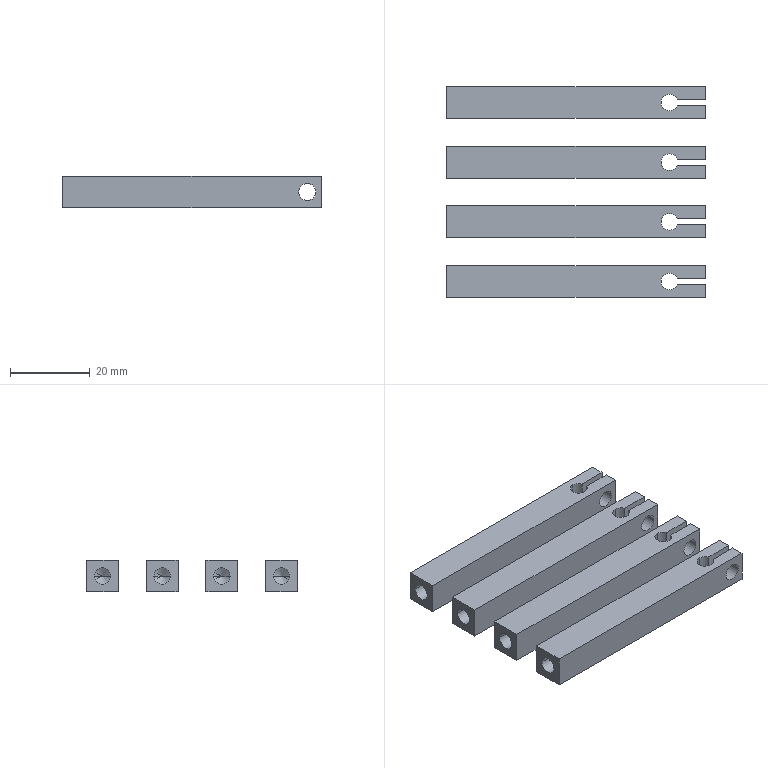NC program | NX | posted with a generic post | part box 65 x 53 x 8 mm
Lines 853 to 3458 of 3458, first 2522 of 2600 lines:
(PLANAR_PROFILE , TOOL : D1.5)
N1692 T13 M6
N1694 G54
N1696 G17 G0 G90 X22.5 Y-34.25 B0. C0. S9500 M3
N1698 G43 Z30. H13
N1700 Z0.9
N1702 G94 G1 Z-0.1 F1000.
N1704 Y-32.5
N1706 Y-25.462
N1708 Y-23.712
N1710 Z0.9
N1712 G0 Z30.
N1714 Z0.8
N1716 G1 Z-0.2
N1718 Y-25.462
N1720 Y-32.5
N1722 Y-34.25
N1724 Z0.8
N1726 G0 Z30.
N1728 Z0.7
N1730 G1 Z-0.3
N1732 Y-32.5
N1734 Y-25.462
N1736 Y-23.712
N1738 Z0.7
N1740 G0 Z30.
N1742 Z0.6
N1744 G1 Z-0.4
N1746 Y-25.462
N1748 Y-32.5
N1750 Y-34.25
N1752 Z0.6
N1754 G0 Z30.
N1756 Z0.5
N1758 G1 Z-0.5
N1760 Y-32.5
N1762 Y-25.462
N1764 Y-23.712
N1766 Z0.5
N1768 G0 Z30.
N1770 Z0.4
N1772 G1 Z-0.6
N1774 Y-25.462
N1776 Y-32.5
N1778 Y-34.25
N1780 Z0.4
N1782 G0 Z30.
N1784 Z0.3
N1786 G1 Z-0.7
N1788 Y-32.5
N1790 Y-25.462
N1792 Y-23.712
N1794 Z0.3
N1796 G0 Z30.
N1798 Z0.2
N1800 G1 Z-0.8
N1802 Y-25.462
N1804 Y-32.5
N1806 Y-34.25
N1808 Z0.2
N1810 G0 Z30.
N1812 Z0.1
N1814 G1 Z-0.9
N1816 Y-32.5
N1818 Y-25.462
N1820 Y-23.712
N1822 Z0.1
N1824 G0 Z30.
N1826 Z0.
N1828 G1 Z-1.
N1830 Y-25.462
N1832 Y-32.5
N1834 Y-34.25
N1836 Z0.
N1838 G0 Z30.
N1840 Z-0.1
N1842 G1 Z-1.1
N1844 Y-32.5
N1846 Y-25.462
N1848 Y-23.712
N1850 Z-0.1
N1852 G0 Z30.
N1854 Z-0.2
N1856 G1 Z-1.2
N1858 Y-25.462
N1860 Y-32.5
N1862 Y-34.25
N1864 Z-0.2
N1866 G0 Z30.
N1868 Z-0.3
N1870 G1 Z-1.3
N1872 Y-32.5
N1874 Y-25.462
N1876 Y-23.712
N1878 Z-0.3
N1880 G0 Z30.
N1882 Z-0.4
N1884 G1 Z-1.4
N1886 Y-25.462
N1888 Y-32.5
N1890 Y-34.25
N1892 Z-0.4
N1894 G0 Z30.
N1896 Z-0.5
N1898 G1 Z-1.5
N1900 Y-32.5
N1902 Y-25.462
N1904 Y-23.712
N1906 Z-0.5
N1908 G0 Z30.
N1910 Z-0.6
N1912 G1 Z-1.6
N1914 Y-25.462
N1916 Y-32.5
N1918 Y-34.25
N1920 Z-0.6
N1922 G0 Z30.
N1924 Z-0.7
N1926 G1 Z-1.7
N1928 Y-32.5
N1930 Y-25.462
N1932 Y-23.712
N1934 Z-0.7
N1936 G0 Z30.
N1938 Z-0.8
N1940 G1 Z-1.8
N1942 Y-25.462
N1944 Y-32.5
N1946 Y-34.25
N1948 Z-0.8
N1950 G0 Z30.
N1952 Z-0.9
N1954 G1 Z-1.9
N1956 Y-32.5
N1958 Y-25.462
N1960 Y-23.712
N1962 Z-0.9
N1964 G0 Z30.
N1966 Z-1.
N1968 G1 Z-2.
N1970 Y-25.462
N1972 Y-32.5
N1974 Y-34.25
N1976 Z-1.
N1978 G0 Z30.
N1980 Z-1.1
N1982 G1 Z-2.1
N1984 Y-32.5
N1986 Y-25.462
N1988 Y-23.712
N1990 Z-1.1
N1992 G0 Z30.
N1994 Z-1.2
N1996 G1 Z-2.2
N1998 Y-25.462
N2000 Y-32.5
N2002 Y-34.25
N2004 Z-1.2
N2006 G0 Z30.
N2008 Z-1.3
N2010 G1 Z-2.3
N2012 Y-32.5
N2014 Y-25.462
N2016 Y-23.712
N2018 Z-1.3
N2020 G0 Z30.
N2022 Z-1.4
N2024 G1 Z-2.4
N2026 Y-25.462
N2028 Y-32.5
N2030 Y-34.25
N2032 Z-1.4
N2034 G0 Z30.
N2036 Z-1.5
N2038 G1 Z-2.5
N2040 Y-32.5
N2042 Y-25.462
N2044 Y-23.712
N2046 Z-1.5
N2048 G0 Z30.
N2050 Z-1.6
N2052 G1 Z-2.6
N2054 Y-25.462
N2056 Y-32.5
N2058 Y-34.25
N2060 Z-1.6
N2062 G0 Z30.
N2064 Z-1.7
N2066 G1 Z-2.7
N2068 Y-32.5
N2070 Y-25.462
N2072 Y-23.712
N2074 Z-1.7
N2076 G0 Z30.
N2078 Z-1.8
N2080 G1 Z-2.8
N2082 Y-25.462
N2084 Y-32.5
N2086 Y-34.25
N2088 Z-1.8
N2090 G0 Z30.
N2092 Z-1.9
N2094 G1 Z-2.9
N2096 Y-32.5
N2098 Y-25.462
N2100 Y-23.712
N2102 Z-1.9
N2104 G0 Z30.
N2106 Z-2.
N2108 G1 Z-3.
N2110 Y-25.462
N2112 Y-32.5
N2114 Y-34.25
N2116 Z-2.
N2118 G0 Z30.
N2120 Z-2.1
N2122 G1 Z-3.1
N2124 Y-32.5
N2126 Y-25.462
N2128 Y-23.712
N2130 Z-2.1
N2132 G0 Z30.
N2134 Z-2.2
N2136 G1 Z-3.2
N2138 Y-25.462
N2140 Y-32.5
N2142 Y-34.25
N2144 Z-2.2
N2146 G0 Z30.
N2148 Z-2.3
N2150 G1 Z-3.3
N2152 Y-32.5
N2154 Y-25.462
N2156 Y-23.712
N2158 Z-2.3
N2160 G0 Z30.
N2162 Z-2.4
N2164 G1 Z-3.4
N2166 Y-25.462
N2168 Y-32.5
N2170 Y-34.25
N2172 Z-2.4
N2174 G0 Z30.
N2176 Z-2.5
N2178 G1 Z-3.5
N2180 Y-32.5
N2182 Y-25.462
N2184 Y-23.712
N2186 Z-2.5
N2188 G0 Z30.
N2190 Z-2.6
N2192 G1 Z-3.6
N2194 Y-25.462
N2196 Y-32.5
N2198 Y-34.25
N2200 Z-2.6
N2202 G0 Z30.
N2204 Z-2.7
N2206 G1 Z-3.7
N2208 Y-32.5
N2210 Y-25.462
N2212 Y-23.712
N2214 Z-2.7
N2216 G0 Z30.
N2218 Z-2.8
N2220 G1 Z-3.8
N2222 Y-25.462
N2224 Y-32.5
N2226 Y-34.25
N2228 Z-2.8
N2230 G0 Z30.
N2232 Z-2.9
N2234 G1 Z-3.9
N2236 Y-32.5
N2238 Y-25.462
N2240 Y-23.712
N2242 Z-2.9
N2244 G0 Z30.
N2246 Z-3.
N2248 G1 Z-4.
N2250 Y-25.462
N2252 Y-32.5
N2254 Y-34.25
N2256 Z-3.
N2258 G0 Z30.
N2260 Z-3.1
N2262 G1 Z-4.1
N2264 Y-32.5
N2266 Y-25.462
N2268 Y-23.712
N2270 Z-3.1
N2272 G0 Z30.
N2274 Z-3.2
N2276 G1 Z-4.2
N2278 Y-25.462
N2280 Y-32.5
N2282 Y-34.25
N2284 Z-3.2
N2286 G0 Z30.
N2288 Z-3.3
N2290 G1 Z-4.3
N2292 Y-32.5
N2294 Y-25.462
N2296 Y-23.712
N2298 Z-3.3
N2300 G0 Z30.
N2302 Z-3.4
N2304 G1 Z-4.4
N2306 Y-25.462
N2308 Y-32.5
N2310 Y-34.25
N2312 Z-3.4
N2314 G0 Z30.
N2316 Z-3.5
N2318 G1 Z-4.5
N2320 Y-32.5
N2322 Y-25.462
N2324 Y-23.712
N2326 Z-3.5
N2328 G0 Z30.
N2330 Z-3.6
N2332 G1 Z-4.6
N2334 Y-25.462
N2336 Y-32.5
N2338 Y-34.25
N2340 Z-3.6
N2342 G0 Z30.
N2344 Z-3.7
N2346 G1 Z-4.7
N2348 Y-32.5
N2350 Y-25.462
N2352 Y-23.712
N2354 Z-3.7
N2356 G0 Z30.
N2358 Z-3.8
N2360 G1 Z-4.8
N2362 Y-25.462
N2364 Y-32.5
N2366 Y-34.25
N2368 Z-3.8
N2370 G0 Z30.
N2372 Z-3.9
N2374 G1 Z-4.9
N2376 Y-32.5
N2378 Y-25.462
N2380 Y-23.712
N2382 Z-3.9
N2384 G0 Z30.
N2386 Z-4.
N2388 G1 Z-5.
N2390 Y-25.462
N2392 Y-32.5
N2394 Y-34.25
N2396 Z-4.
N2398 G0 Z30.
N2400 Z-4.1
N2402 G1 Z-5.1
N2404 Y-32.5
N2406 Y-25.462
N2408 Y-23.712
N2410 Z-4.1
N2412 G0 Z30.
N2414 Z-4.2
N2416 G1 Z-5.2
N2418 Y-25.462
N2420 Y-32.5
N2422 Y-34.25
N2424 Z-4.2
N2426 G0 Z30.
N2428 Z-4.3
N2430 G1 Z-5.3
N2432 Y-32.5
N2434 Y-25.462
N2436 Y-23.712
N2438 Z-4.3
N2440 G0 Z30.
N2442 Z-4.4
N2444 G1 Z-5.4
N2446 Y-25.462
N2448 Y-32.5
N2450 Y-34.25
N2452 Z-4.4
N2454 G0 Z30.
N2456 Z-4.5
N2458 G1 Z-5.5
N2460 Y-32.5
N2462 Y-25.462
N2464 Y-23.712
N2466 Z-4.5
N2468 G0 Z30.
N2470 Z-4.6
N2472 G1 Z-5.6
N2474 Y-25.462
N2476 Y-32.5
N2478 Y-34.25
N2480 Z-4.6
N2482 G0 Z30.
N2484 Z-4.7
N2486 G1 Z-5.7
N2488 Y-32.5
N2490 Y-25.462
N2492 Y-23.712
N2494 Z-4.7
N2496 G0 Z30.
N2498 Z-4.8
N2500 G1 Z-5.8
N2502 Y-25.462
N2504 Y-32.5
N2506 Y-34.25
N2508 Z-4.8
N2510 G0 Z30.
N2512 Z-4.9
N2514 G1 Z-5.9
N2516 Y-32.5
N2518 Y-25.462
N2520 Y-23.712
N2522 Z-4.9
N2524 G0 Z30.
N2526 Z-5.
N2528 G1 Z-6.
N2530 Y-25.462
N2532 Y-32.5
N2534 Y-34.25
N2536 Z-5.
N2538 G0 Z30.
N2540 Z-5.1
N2542 G1 Z-6.1
N2544 Y-32.5
N2546 Y-25.462
N2548 Y-23.712
N2550 Z-5.1
N2552 G0 Z30.
N2554 Z-5.2
N2556 G1 Z-6.2
N2558 Y-25.462
N2560 Y-32.5
N2562 Y-34.25
N2564 Z-5.2
N2566 G0 Z30.
N2568 Z-5.3
N2570 G1 Z-6.3
N2572 Y-32.5
N2574 Y-25.462
N2576 Y-23.712
N2578 Z-5.3
N2580 G0 Z30.
N2582 Z-5.4
N2584 G1 Z-6.4
N2586 Y-25.462
N2588 Y-32.5
N2590 Y-34.25
N2592 Z-5.4
N2594 G0 Z30.
N2596 Z-5.5
N2598 G1 Z-6.5
N2600 Y-32.5
N2602 Y-25.462
N2604 Y-23.712
N2606 Z-5.5
N2608 G0 Z30.
N2610 Z-5.6
N2612 G1 Z-6.6
N2614 Y-25.462
N2616 Y-32.5
N2618 Y-34.25
N2620 Z-5.6
N2622 G0 Z30.
N2624 Z-5.7
N2626 G1 Z-6.7
N2628 Y-32.5
N2630 Y-25.462
N2632 Y-23.712
N2634 Z-5.7
N2636 G0 Z30.
N2638 Z-5.8
N2640 G1 Z-6.8
N2642 Y-25.462
N2644 Y-32.5
N2646 Y-34.25
N2648 Z-5.8
N2650 G0 Z30.
N2652 Z-5.9
N2654 G1 Z-6.9
N2656 Y-32.5
N2658 Y-25.462
N2660 Y-23.712
N2662 Z-5.9
N2664 G0 Z30.
N2666 Z-6.
N2668 G1 Z-7.
N2670 Y-25.462
N2672 Y-32.5
N2674 Y-34.25
N2676 Z-6.
N2678 G0 Z30.
N2680 Z-6.1
N2682 G1 Z-7.1
N2684 Y-32.5
N2686 Y-25.462
N2688 Y-23.712
N2690 Z-6.1
N2692 G0 Z30.
N2694 Z-6.2
N2696 G1 Z-7.2
N2698 Y-25.462
N2700 Y-32.5
N2702 Y-34.25
N2704 Z-6.2
N2706 G0 Z30.
N2708 Z-6.3
N2710 G1 Z-7.3
N2712 Y-32.5
N2714 Y-25.462
N2716 Y-23.712
N2718 Z-6.3
N2720 G0 Z30.
N2722 Z-6.4
N2724 G1 Z-7.4
N2726 Y-25.462
N2728 Y-32.5
N2730 Y-34.25
N2732 Z-6.4
N2734 G0 Z30.
N2736 Z-6.5
N2738 G1 Z-7.5
N2740 Y-32.5
N2742 Y-25.462
N2744 Y-23.712
N2746 Z-6.5
N2748 G0 Z30.
N2750 Z-6.6
N2752 G1 Z-7.6
N2754 Y-25.462
N2756 Y-32.5
N2758 Y-34.25
N2760 Z-6.6
N2762 G0 Z30.
N2764 Z-6.7
N2766 G1 Z-7.7
N2768 Y-32.5
N2770 Y-25.462
N2772 Y-23.712
N2774 Z-6.7
N2776 G0 Z30.
N2778 Z-6.8
N2780 G1 Z-7.8
N2782 Y-25.462
N2784 Y-32.5
N2786 Y-34.25
N2788 Z-6.8
N2790 G0 Z30.
N2792 Z-6.9
N2794 G1 Z-7.9
N2796 Y-32.5
N2798 Y-25.462
N2800 Y-23.712
N2802 Z-6.9
N2804 G0 Z30.
N2806 Z-7.
N2808 G1 Z-8.
N2810 Y-25.462
N2812 Y-32.5
N2814 Y-34.25
N2816 Z-7.
N2818 G0 Z30.
N2820 X7.5
N2822 Z0.9
N2824 G1 Z-0.1
N2826 Y-32.5
N2828 Y-25.462
N2830 Y-23.712
N2832 Z0.9
N2834 G0 Z30.
N2836 Z0.8
N2838 G1 Z-0.2
N2840 Y-25.462
N2842 Y-32.5
N2844 Y-34.25
N2846 Z0.8
N2848 G0 Z30.
N2850 Z0.7
N2852 G1 Z-0.3
N2854 Y-32.5
N2856 Y-25.462
N2858 Y-23.712
N2860 Z0.7
N2862 G0 Z30.
N2864 Z0.6
N2866 G1 Z-0.4
N2868 Y-25.462
N2870 Y-32.5
N2872 Y-34.25
N2874 Z0.6
N2876 G0 Z30.
N2878 Z0.5
N2880 G1 Z-0.5
N2882 Y-32.5
N2884 Y-25.462
N2886 Y-23.712
N2888 Z0.5
N2890 G0 Z30.
N2892 Z0.4
N2894 G1 Z-0.6
N2896 Y-25.462
N2898 Y-32.5
N2900 Y-34.25
N2902 Z0.4
N2904 G0 Z30.
N2906 Z0.3
N2908 G1 Z-0.7
N2910 Y-32.5
N2912 Y-25.462
N2914 Y-23.712
N2916 Z0.3
N2918 G0 Z30.
N2920 Z0.2
N2922 G1 Z-0.8
N2924 Y-25.462
N2926 Y-32.5
N2928 Y-34.25
N2930 Z0.2
N2932 G0 Z30.
N2934 Z0.1
N2936 G1 Z-0.9
N2938 Y-32.5
N2940 Y-25.462
N2942 Y-23.712
N2944 Z0.1
N2946 G0 Z30.
N2948 Z0.
N2950 G1 Z-1.
N2952 Y-25.462
N2954 Y-32.5
N2956 Y-34.25
N2958 Z0.
N2960 G0 Z30.
N2962 Z-0.1
N2964 G1 Z-1.1
N2966 Y-32.5
N2968 Y-25.462
N2970 Y-23.712
N2972 Z-0.1
N2974 G0 Z30.
N2976 Z-0.2
N2978 G1 Z-1.2
N2980 Y-25.462
N2982 Y-32.5
N2984 Y-34.25
N2986 Z-0.2
N2988 G0 Z30.
N2990 Z-0.3
N2992 G1 Z-1.3
N2994 Y-32.5
N2996 Y-25.462
N2998 Y-23.712
N3000 Z-0.3
N3002 G0 Z30.
N3004 Z-0.4
N3006 G1 Z-1.4
N3008 Y-25.462
N3010 Y-32.5
N3012 Y-34.25
N3014 Z-0.4
N3016 G0 Z30.
N3018 Z-0.5
N3020 G1 Z-1.5
N3022 Y-32.5
N3024 Y-25.462
N3026 Y-23.712
N3028 Z-0.5
N3030 G0 Z30.
N3032 Z-0.6
N3034 G1 Z-1.6
N3036 Y-25.462
N3038 Y-32.5
N3040 Y-34.25
N3042 Z-0.6
N3044 G0 Z30.
N3046 Z-0.7
N3048 G1 Z-1.7
N3050 Y-32.5
N3052 Y-25.462
N3054 Y-23.712
N3056 Z-0.7
N3058 G0 Z30.
N3060 Z-0.8
N3062 G1 Z-1.8
N3064 Y-25.462
N3066 Y-32.5
N3068 Y-34.25
N3070 Z-0.8
N3072 G0 Z30.
N3074 Z-0.9
N3076 G1 Z-1.9
N3078 Y-32.5
N3080 Y-25.462
N3082 Y-23.712
N3084 Z-0.9
N3086 G0 Z30.
N3088 Z-1.
N3090 G1 Z-2.
N3092 Y-25.462
N3094 Y-32.5
N3096 Y-34.25
N3098 Z-1.
N3100 G0 Z30.
N3102 Z-1.1
N3104 G1 Z-2.1
N3106 Y-32.5
N3108 Y-25.462
N3110 Y-23.712
N3112 Z-1.1
N3114 G0 Z30.
N3116 Z-1.2
N3118 G1 Z-2.2
N3120 Y-25.462
N3122 Y-32.5
N3124 Y-34.25
N3126 Z-1.2
N3128 G0 Z30.
N3130 Z-1.3
N3132 G1 Z-2.3
N3134 Y-32.5
N3136 Y-25.462
N3138 Y-23.712
N3140 Z-1.3
N3142 G0 Z30.
N3144 Z-1.4
N3146 G1 Z-2.4
N3148 Y-25.462
N3150 Y-32.5
N3152 Y-34.25
N3154 Z-1.4
N3156 G0 Z30.
N3158 Z-1.5
N3160 G1 Z-2.5
N3162 Y-32.5
N3164 Y-25.462
N3166 Y-23.712
N3168 Z-1.5
N3170 G0 Z30.
N3172 Z-1.6
N3174 G1 Z-2.6
N3176 Y-25.462
N3178 Y-32.5
N3180 Y-34.25
N3182 Z-1.6
N3184 G0 Z30.
N3186 Z-1.7
N3188 G1 Z-2.7
N3190 Y-32.5
N3192 Y-25.462
N3194 Y-23.712
N3196 Z-1.7
N3198 G0 Z30.
N3200 Z-1.8
N3202 G1 Z-2.8
N3204 Y-25.462
N3206 Y-32.5
N3208 Y-34.25
N3210 Z-1.8
N3212 G0 Z30.
N3214 Z-1.9
N3216 G1 Z-2.9
N3218 Y-32.5
N3220 Y-25.462
N3222 Y-23.712
N3224 Z-1.9
N3226 G0 Z30.
N3228 Z-2.
N3230 G1 Z-3.
N3232 Y-25.462
N3234 Y-32.5
N3236 Y-34.25
N3238 Z-2.
N3240 G0 Z30.
N3242 Z-2.1
N3244 G1 Z-3.1
N3246 Y-32.5
N3248 Y-25.462
N3250 Y-23.712
N3252 Z-2.1
N3254 G0 Z30.
N3256 Z-2.2
N3258 G1 Z-3.2
N3260 Y-25.462
N3262 Y-32.5
N3264 Y-34.25
N3266 Z-2.2
N3268 G0 Z30.
N3270 Z-2.3
N3272 G1 Z-3.3
N3274 Y-32.5
N3276 Y-25.462
N3278 Y-23.712
N3280 Z-2.3
N3282 G0 Z30.
N3284 Z-2.4
N3286 G1 Z-3.4
N3288 Y-25.462
N3290 Y-32.5
N3292 Y-34.25
N3294 Z-2.4
N3296 G0 Z30.
N3298 Z-2.5
N3300 G1 Z-3.5
N3302 Y-32.5
N3304 Y-25.462
N3306 Y-23.712
N3308 Z-2.5
N3310 G0 Z30.
N3312 Z-2.6
N3314 G1 Z-3.6
N3316 Y-25.462
N3318 Y-32.5
N3320 Y-34.25
N3322 Z-2.6
N3324 G0 Z30.
N3326 Z-2.7
N3328 G1 Z-3.7
N3330 Y-32.5
N3332 Y-25.462
N3334 Y-23.712
N3336 Z-2.7
N3338 G0 Z30.
N3340 Z-2.8
N3342 G1 Z-3.8
N3344 Y-25.462
N3346 Y-32.5
N3348 Y-34.25
N3350 Z-2.8
N3352 G0 Z30.
N3354 Z-2.9
N3356 G1 Z-3.9
N3358 Y-32.5
N3360 Y-25.462
N3362 Y-23.712
N3364 Z-2.9
N3366 G0 Z30.
N3368 Z-3.
N3370 G1 Z-4.
N3372 Y-25.462
N3374 Y-32.5
N3376 Y-34.25
N3378 Z-3.
N3380 G0 Z30.
N3382 Z-3.1
N3384 G1 Z-4.1
N3386 Y-32.5
N3388 Y-25.462
N3390 Y-23.712
N3392 Z-3.1
N3394 G0 Z30.
N3396 Z-3.2
N3398 G1 Z-4.2
N3400 Y-25.462
N3402 Y-32.5
N3404 Y-34.25
N3406 Z-3.2
N3408 G0 Z30.
N3410 Z-3.3
N3412 G1 Z-4.3
N3414 Y-32.5
N3416 Y-25.462
N3418 Y-23.712
N3420 Z-3.3
N3422 G0 Z30.
N3424 Z-3.4
N3426 G1 Z-4.4
N3428 Y-25.462
N3430 Y-32.5
N3432 Y-34.25
N3434 Z-3.4
N3436 G0 Z30.
N3438 Z-3.5
N3440 G1 Z-4.5
N3442 Y-32.5
N3444 Y-25.462
N3446 Y-23.712
N3448 Z-3.5
N3450 G0 Z30.
N3452 Z-3.6
N3454 G1 Z-4.6
N3456 Y-25.462
N3458 Y-32.5
N3460 Y-34.25
N3462 Z-3.6
N3464 G0 Z30.
N3466 Z-3.7
N3468 G1 Z-4.7
N3470 Y-32.5
N3472 Y-25.462
N3474 Y-23.712
N3476 Z-3.7
N3478 G0 Z30.
N3480 Z-3.8
N3482 G1 Z-4.8
N3484 Y-25.462
N3486 Y-32.5
N3488 Y-34.25
N3490 Z-3.8
N3492 G0 Z30.
N3494 Z-3.9
N3496 G1 Z-4.9
N3498 Y-32.5
N3500 Y-25.462
N3502 Y-23.712
N3504 Z-3.9
N3506 G0 Z30.
N3508 Z-4.
N3510 G1 Z-5.
N3512 Y-25.462
N3514 Y-32.5
N3516 Y-34.25
N3518 Z-4.
N3520 G0 Z30.
N3522 Z-4.1
N3524 G1 Z-5.1
N3526 Y-32.5
N3528 Y-25.462
N3530 Y-23.712
N3532 Z-4.1
N3534 G0 Z30.
N3536 Z-4.2
N3538 G1 Z-5.2
N3540 Y-25.462
N3542 Y-32.5
N3544 Y-34.25
N3546 Z-4.2
N3548 G0 Z30.
N3550 Z-4.3
N3552 G1 Z-5.3
N3554 Y-32.5
N3556 Y-25.462
N3558 Y-23.712
N3560 Z-4.3
N3562 G0 Z30.
N3564 Z-4.4
N3566 G1 Z-5.4
N3568 Y-25.462
N3570 Y-32.5
N3572 Y-34.25
N3574 Z-4.4
N3576 G0 Z30.
N3578 Z-4.5
N3580 G1 Z-5.5
N3582 Y-32.5
N3584 Y-25.462
N3586 Y-23.712
N3588 Z-4.5
N3590 G0 Z30.
N3592 Z-4.6
N3594 G1 Z-5.6
N3596 Y-25.462
N3598 Y-32.5
N3600 Y-34.25
N3602 Z-4.6
N3604 G0 Z30.
N3606 Z-4.7
N3608 G1 Z-5.7
N3610 Y-32.5
N3612 Y-25.462
N3614 Y-23.712
N3616 Z-4.7
N3618 G0 Z30.
N3620 Z-4.8
N3622 G1 Z-5.8
N3624 Y-25.462
N3626 Y-32.5
N3628 Y-34.25
N3630 Z-4.8
N3632 G0 Z30.
N3634 Z-4.9
N3636 G1 Z-5.9
N3638 Y-32.5
N3640 Y-25.462
N3642 Y-23.712
N3644 Z-4.9
N3646 G0 Z30.
N3648 Z-5.
N3650 G1 Z-6.
N3652 Y-25.462
N3654 Y-32.5
N3656 Y-34.25
N3658 Z-5.
N3660 G0 Z30.
N3662 Z-5.1
N3664 G1 Z-6.1
N3666 Y-32.5
N3668 Y-25.462
N3670 Y-23.712
N3672 Z-5.1
N3674 G0 Z30.
N3676 Z-5.2
N3678 G1 Z-6.2
N3680 Y-25.462
N3682 Y-32.5
N3684 Y-34.25
N3686 Z-5.2
N3688 G0 Z30.
N3690 Z-5.3
N3692 G1 Z-6.3
N3694 Y-32.5
N3696 Y-25.462
N3698 Y-23.712
N3700 Z-5.3
N3702 G0 Z30.
N3704 Z-5.4
N3706 G1 Z-6.4
N3708 Y-25.462
N3710 Y-32.5
N3712 Y-34.25
N3714 Z-5.4
N3716 G0 Z30.
N3718 Z-5.5
N3720 G1 Z-6.5
N3722 Y-32.5
N3724 Y-25.462
N3726 Y-23.712
N3728 Z-5.5
N3730 G0 Z30.
N3732 Z-5.6
N3734 G1 Z-6.6
N3736 Y-25.462
N3738 Y-32.5
N3740 Y-34.25
N3742 Z-5.6
N3744 G0 Z30.
N3746 Z-5.7
N3748 G1 Z-6.7
N3750 Y-32.5
N3752 Y-25.462
N3754 Y-23.712
N3756 Z-5.7
N3758 G0 Z30.
N3760 Z-5.8
N3762 G1 Z-6.8
N3764 Y-25.462
N3766 Y-32.5
N3768 Y-34.25
N3770 Z-5.8
N3772 G0 Z30.
N3774 Z-5.9
N3776 G1 Z-6.9
N3778 Y-32.5
N3780 Y-25.462
N3782 Y-23.712
N3784 Z-5.9
N3786 G0 Z30.
N3788 Z-6.
N3790 G1 Z-7.
N3792 Y-25.462
N3794 Y-32.5
N3796 Y-34.25
N3798 Z-6.
N3800 G0 Z30.
N3802 Z-6.1
N3804 G1 Z-7.1
N3806 Y-32.5
N3808 Y-25.462
N3810 Y-23.712
N3812 Z-6.1
N3814 G0 Z30.
N3816 Z-6.2
N3818 G1 Z-7.2
N3820 Y-25.462
N3822 Y-32.5
N3824 Y-34.25
N3826 Z-6.2
N3828 G0 Z30.
N3830 Z-6.3
N3832 G1 Z-7.3
N3834 Y-32.5
N3836 Y-25.462
N3838 Y-23.712
N3840 Z-6.3
N3842 G0 Z30.
N3844 Z-6.4
N3846 G1 Z-7.4
N3848 Y-25.462
N3850 Y-32.5
N3852 Y-34.25
N3854 Z-6.4
N3856 G0 Z30.
N3858 Z-6.5
N3860 G1 Z-7.5
N3862 Y-32.5
N3864 Y-25.462
N3866 Y-23.712
N3868 Z-6.5
N3870 G0 Z30.
N3872 Z-6.6
N3874 G1 Z-7.6
N3876 Y-25.462
N3878 Y-32.5
N3880 Y-34.25
N3882 Z-6.6
N3884 G0 Z30.
N3886 Z-6.7
N3888 G1 Z-7.7
N3890 Y-32.5
N3892 Y-25.462
N3894 Y-23.712
N3896 Z-6.7
N3898 G0 Z30.
N3900 Z-6.8
N3902 G1 Z-7.8
N3904 Y-25.462
N3906 Y-32.5
N3908 Y-34.25
N3910 Z-6.8
N3912 G0 Z30.
N3914 Z-6.9
N3916 G1 Z-7.9
N3918 Y-32.5
N3920 Y-25.462
N3922 Y-23.712
N3924 Z-6.9
N3926 G0 Z30.
N3928 Z-7.
N3930 G1 Z-8.
N3932 Y-25.462
N3934 Y-32.5
N3936 Y-34.25
N3938 Z-7.
N3940 G0 Z30.
N3942 X-7.5
N3944 Z0.9
N3946 G1 Z-0.1
N3948 Y-32.5
N3950 Y-25.462
N3952 Y-23.712
N3954 Z0.9
N3956 G0 Z30.
N3958 Z0.8
N3960 G1 Z-0.2
N3962 Y-25.462
N3964 Y-32.5
N3966 Y-34.25
N3968 Z0.8
N3970 G0 Z30.
N3972 Z0.7
N3974 G1 Z-0.3
N3976 Y-32.5
N3978 Y-25.462
N3980 Y-23.712
N3982 Z0.7
N3984 G0 Z30.
N3986 Z0.6
N3988 G1 Z-0.4
N3990 Y-25.462
N3992 Y-32.5
N3994 Y-34.25
N3996 Z0.6
N3998 G0 Z30.
N4000 Z0.5
N4002 G1 Z-0.5
N4004 Y-32.5
N4006 Y-25.462
N4008 Y-23.712
N4010 Z0.5
N4012 G0 Z30.
N4014 Z0.4
N4016 G1 Z-0.6
N4018 Y-25.462
N4020 Y-32.5
N4022 Y-34.25
N4024 Z0.4
N4026 G0 Z30.
N4028 Z0.3
N4030 G1 Z-0.7
N4032 Y-32.5
N4034 Y-25.462
N4036 Y-23.712
N4038 Z0.3
N4040 G0 Z30.
N4042 Z0.2
N4044 G1 Z-0.8
N4046 Y-25.462
N4048 Y-32.5
N4050 Y-34.25
N4052 Z0.2
N4054 G0 Z30.
N4056 Z0.1
N4058 G1 Z-0.9
N4060 Y-32.5
N4062 Y-25.462
N4064 Y-23.712
N4066 Z0.1
N4068 G0 Z30.
N4070 Z0.
N4072 G1 Z-1.
N4074 Y-25.462
N4076 Y-32.5
N4078 Y-34.25
N4080 Z0.
N4082 G0 Z30.
N4084 Z-0.1
N4086 G1 Z-1.1
N4088 Y-32.5
N4090 Y-25.462
N4092 Y-23.712
N4094 Z-0.1
N4096 G0 Z30.
N4098 Z-0.2
N4100 G1 Z-1.2
N4102 Y-25.462
N4104 Y-32.5
N4106 Y-34.25
N4108 Z-0.2
N4110 G0 Z30.
N4112 Z-0.3
N4114 G1 Z-1.3
N4116 Y-32.5
N4118 Y-25.462
N4120 Y-23.712
N4122 Z-0.3
N4124 G0 Z30.
N4126 Z-0.4
N4128 G1 Z-1.4
N4130 Y-25.462
N4132 Y-32.5
N4134 Y-34.25
N4136 Z-0.4
N4138 G0 Z30.
N4140 Z-0.5
N4142 G1 Z-1.5
N4144 Y-32.5
N4146 Y-25.462
N4148 Y-23.712
N4150 Z-0.5
N4152 G0 Z30.
N4154 Z-0.6
N4156 G1 Z-1.6
N4158 Y-25.462
N4160 Y-32.5
N4162 Y-34.25
N4164 Z-0.6
N4166 G0 Z30.
N4168 Z-0.7
N4170 G1 Z-1.7
N4172 Y-32.5
N4174 Y-25.462
N4176 Y-23.712
N4178 Z-0.7
N4180 G0 Z30.
N4182 Z-0.8
N4184 G1 Z-1.8
N4186 Y-25.462
N4188 Y-32.5
N4190 Y-34.25
N4192 Z-0.8
N4194 G0 Z30.
N4196 Z-0.9
N4198 G1 Z-1.9
N4200 Y-32.5
N4202 Y-25.462
N4204 Y-23.712
N4206 Z-0.9
N4208 G0 Z30.
N4210 Z-1.
N4212 G1 Z-2.
N4214 Y-25.462
N4216 Y-32.5
N4218 Y-34.25
N4220 Z-1.
N4222 G0 Z30.
N4224 Z-1.1
N4226 G1 Z-2.1
N4228 Y-32.5
N4230 Y-25.462
N4232 Y-23.712
N4234 Z-1.1
N4236 G0 Z30.
N4238 Z-1.2
N4240 G1 Z-2.2
N4242 Y-25.462
N4244 Y-32.5
N4246 Y-34.25
N4248 Z-1.2
N4250 G0 Z30.
N4252 Z-1.3
N4254 G1 Z-2.3
N4256 Y-32.5
N4258 Y-25.462
N4260 Y-23.712
N4262 Z-1.3
N4264 G0 Z30.
N4266 Z-1.4
N4268 G1 Z-2.4
N4270 Y-25.462
N4272 Y-32.5
N4274 Y-34.25
N4276 Z-1.4
N4278 G0 Z30.
N4280 Z-1.5
N4282 G1 Z-2.5
N4284 Y-32.5
N4286 Y-25.462
N4288 Y-23.712
N4290 Z-1.5
N4292 G0 Z30.
N4294 Z-1.6
N4296 G1 Z-2.6
N4298 Y-25.462
N4300 Y-32.5
N4302 Y-34.25
N4304 Z-1.6
N4306 G0 Z30.
N4308 Z-1.7
N4310 G1 Z-2.7
N4312 Y-32.5
N4314 Y-25.462
N4316 Y-23.712
N4318 Z-1.7
N4320 G0 Z30.
N4322 Z-1.8
N4324 G1 Z-2.8
N4326 Y-25.462
N4328 Y-32.5
N4330 Y-34.25
N4332 Z-1.8
N4334 G0 Z30.
N4336 Z-1.9
N4338 G1 Z-2.9
N4340 Y-32.5
N4342 Y-25.462
N4344 Y-23.712
N4346 Z-1.9
N4348 G0 Z30.
N4350 Z-2.
N4352 G1 Z-3.
N4354 Y-25.462
N4356 Y-32.5
N4358 Y-34.25
N4360 Z-2.
N4362 G0 Z30.
N4364 Z-2.1
N4366 G1 Z-3.1
N4368 Y-32.5
N4370 Y-25.462
N4372 Y-23.712
N4374 Z-2.1
N4376 G0 Z30.
N4378 Z-2.2
N4380 G1 Z-3.2
N4382 Y-25.462
N4384 Y-32.5
N4386 Y-34.25
N4388 Z-2.2
N4390 G0 Z30.
N4392 Z-2.3
N4394 G1 Z-3.3
N4396 Y-32.5
N4398 Y-25.462
N4400 Y-23.712
N4402 Z-2.3
N4404 G0 Z30.
N4406 Z-2.4
N4408 G1 Z-3.4
N4410 Y-25.462
N4412 Y-32.5
N4414 Y-34.25
N4416 Z-2.4
N4418 G0 Z30.
N4420 Z-2.5
N4422 G1 Z-3.5
N4424 Y-32.5
N4426 Y-25.462
N4428 Y-23.712
N4430 Z-2.5
N4432 G0 Z30.
N4434 Z-2.6
N4436 G1 Z-3.6
N4438 Y-25.462
N4440 Y-32.5
N4442 Y-34.25
N4444 Z-2.6
N4446 G0 Z30.
N4448 Z-2.7
N4450 G1 Z-3.7
N4452 Y-32.5
N4454 Y-25.462
N4456 Y-23.712
N4458 Z-2.7
N4460 G0 Z30.
N4462 Z-2.8
N4464 G1 Z-3.8
N4466 Y-25.462
N4468 Y-32.5
N4470 Y-34.25
N4472 Z-2.8
N4474 G0 Z30.
N4476 Z-2.9
N4478 G1 Z-3.9
N4480 Y-32.5
N4482 Y-25.462
N4484 Y-23.712
N4486 Z-2.9
N4488 G0 Z30.
N4490 Z-3.
N4492 G1 Z-4.
N4494 Y-25.462
N4496 Y-32.5
N4498 Y-34.25
N4500 Z-3.
N4502 G0 Z30.
N4504 Z-3.1
N4506 G1 Z-4.1
N4508 Y-32.5
N4510 Y-25.462
N4512 Y-23.712
N4514 Z-3.1
N4516 G0 Z30.
N4518 Z-3.2
N4520 G1 Z-4.2
N4522 Y-25.462
N4524 Y-32.5
N4526 Y-34.25
N4528 Z-3.2
N4530 G0 Z30.
N4532 Z-3.3
N4534 G1 Z-4.3
N4536 Y-32.5
N4538 Y-25.462
N4540 Y-23.712
N4542 Z-3.3
N4544 G0 Z30.
N4546 Z-3.4
N4548 G1 Z-4.4
N4550 Y-25.462
N4552 Y-32.5
N4554 Y-34.25
N4556 Z-3.4
N4558 G0 Z30.
N4560 Z-3.5
N4562 G1 Z-4.5
N4564 Y-32.5
N4566 Y-25.462
N4568 Y-23.712
N4570 Z-3.5
N4572 G0 Z30.
N4574 Z-3.6
N4576 G1 Z-4.6
N4578 Y-25.462
N4580 Y-32.5
N4582 Y-34.25
N4584 Z-3.6
N4586 G0 Z30.
N4588 Z-3.7
N4590 G1 Z-4.7
N4592 Y-32.5
N4594 Y-25.462
N4596 Y-23.712
N4598 Z-3.7
N4600 G0 Z30.
N4602 Z-3.8
N4604 G1 Z-4.8
N4606 Y-25.462
N4608 Y-32.5
N4610 Y-34.25
N4612 Z-3.8
N4614 G0 Z30.
N4616 Z-3.9
N4618 G1 Z-4.9
N4620 Y-32.5
N4622 Y-25.462
N4624 Y-23.712
N4626 Z-3.9
N4628 G0 Z30.
N4630 Z-4.
N4632 G1 Z-5.
N4634 Y-25.462
N4636 Y-32.5
N4638 Y-34.25
N4640 Z-4.
N4642 G0 Z30.
N4644 Z-4.1
N4646 G1 Z-5.1
N4648 Y-32.5
N4650 Y-25.462
N4652 Y-23.712
N4654 Z-4.1
N4656 G0 Z30.
N4658 Z-4.2
N4660 G1 Z-5.2
N4662 Y-25.462
N4664 Y-32.5
N4666 Y-34.25
N4668 Z-4.2
N4670 G0 Z30.
N4672 Z-4.3
N4674 G1 Z-5.3
N4676 Y-32.5
N4678 Y-25.462
N4680 Y-23.712
N4682 Z-4.3
N4684 G0 Z30.
N4686 Z-4.4
N4688 G1 Z-5.4
N4690 Y-25.462
N4692 Y-32.5
N4694 Y-34.25
N4696 Z-4.4
N4698 G0 Z30.
N4700 Z-4.5
N4702 G1 Z-5.5
N4704 Y-32.5
N4706 Y-25.462
N4708 Y-23.712
N4710 Z-4.5
N4712 G0 Z30.
N4714 Z-4.6
N4716 G1 Z-5.6
N4718 Y-25.462
N4720 Y-32.5
N4722 Y-34.25
N4724 Z-4.6
N4726 G0 Z30.
N4728 Z-4.7
N4730 G1 Z-5.7
N4732 Y-32.5
N4734 Y-25.462
N4736 Y-23.712
N4738 Z-4.7
N4740 G0 Z30.
N4742 Z-4.8
N4744 G1 Z-5.8
N4746 Y-25.462
N4748 Y-32.5
N4750 Y-34.25
N4752 Z-4.8
N4754 G0 Z30.
N4756 Z-4.9
N4758 G1 Z-5.9
N4760 Y-32.5
N4762 Y-25.462
N4764 Y-23.712
N4766 Z-4.9
N4768 G0 Z30.
N4770 Z-5.
N4772 G1 Z-6.
N4774 Y-25.462
N4776 Y-32.5
N4778 Y-34.25
N4780 Z-5.
N4782 G0 Z30.
N4784 Z-5.1
N4786 G1 Z-6.1
N4788 Y-32.5
N4790 Y-25.462
N4792 Y-23.712
N4794 Z-5.1
N4796 G0 Z30.
N4798 Z-5.2
N4800 G1 Z-6.2
N4802 Y-25.462
N4804 Y-32.5
N4806 Y-34.25
N4808 Z-5.2
N4810 G0 Z30.
N4812 Z-5.3
N4814 G1 Z-6.3
N4816 Y-32.5
N4818 Y-25.462
N4820 Y-23.712
N4822 Z-5.3
N4824 G0 Z30.
N4826 Z-5.4
N4828 G1 Z-6.4
N4830 Y-25.462
N4832 Y-32.5
N4834 Y-34.25
N4836 Z-5.4
N4838 G0 Z30.
N4840 Z-5.5
N4842 G1 Z-6.5
N4844 Y-32.5
N4846 Y-25.462
N4848 Y-23.712
N4850 Z-5.5
N4852 G0 Z30.
N4854 Z-5.6
N4856 G1 Z-6.6
N4858 Y-25.462
N4860 Y-32.5
N4862 Y-34.25
N4864 Z-5.6
N4866 G0 Z30.
N4868 Z-5.7
N4870 G1 Z-6.7
N4872 Y-32.5
N4874 Y-25.462
N4876 Y-23.712
N4878 Z-5.7
N4880 G0 Z30.
N4882 Z-5.8
N4884 G1 Z-6.8
N4886 Y-25.462
N4888 Y-32.5
N4890 Y-34.25
N4892 Z-5.8
N4894 G0 Z30.
N4896 Z-5.9
N4898 G1 Z-6.9
N4900 Y-32.5
N4902 Y-25.462
N4904 Y-23.712
N4906 Z-5.9
N4908 G0 Z30.
N4910 Z-6.
N4912 G1 Z-7.
N4914 Y-25.462
N4916 Y-32.5
N4918 Y-34.25
N4920 Z-6.
N4922 G0 Z30.
N4924 Z-6.1
N4926 G1 Z-7.1
N4928 Y-32.5
N4930 Y-25.462
N4932 Y-23.712
N4934 Z-6.1
N4936 G0 Z30.
N4938 Z-6.2
N4940 G1 Z-7.2
N4942 Y-25.462
N4944 Y-32.5
N4946 Y-34.25
N4948 Z-6.2
N4950 G0 Z30.
N4952 Z-6.3
N4954 G1 Z-7.3
N4956 Y-32.5
N4958 Y-25.462
N4960 Y-23.712
N4962 Z-6.3
N4964 G0 Z30.
N4966 Z-6.4
N4968 G1 Z-7.4
N4970 Y-25.462
N4972 Y-32.5
N4974 Y-34.25
N4976 Z-6.4
N4978 G0 Z30.
N4980 Z-6.5
N4982 G1 Z-7.5
N4984 Y-32.5
N4986 Y-25.462
N4988 Y-23.712
N4990 Z-6.5
N4992 G0 Z30.
N4994 Z-6.6
N4996 G1 Z-7.6
N4998 Y-25.462
N5000 Y-32.5
N5002 Y-34.25
N5004 Z-6.6
N5006 G0 Z30.
N5008 Z-6.7
N5010 G1 Z-7.7
N5012 Y-32.5
N5014 Y-25.462
N5016 Y-23.712
N5018 Z-6.7
N5020 G0 Z30.
N5022 Z-6.8
N5024 G1 Z-7.8
N5026 Y-25.462
N5028 Y-32.5
N5030 Y-34.25
N5032 Z-6.8
N5034 G0 Z30.
N5036 Z-6.9
N5038 G1 Z-7.9
N5040 Y-32.5
N5042 Y-25.462
N5044 Y-23.712
N5046 Z-6.9
N5048 G0 Z30.
N5050 Z-7.
N5052 G1 Z-8.
N5054 Y-25.462
N5056 Y-32.5
N5058 Y-34.25
N5060 Z-7.
N5062 G0 Z30.
N5064 X-22.5
N5066 Z0.9
N5068 G1 Z-0.1
N5070 Y-32.5
N5072 Y-25.462
N5074 Y-23.712
N5076 Z0.9
N5078 G0 Z30.
N5080 Z0.8
N5082 G1 Z-0.2
N5084 Y-25.462
N5086 Y-32.5
N5088 Y-34.25
N5090 Z0.8
N5092 G0 Z30.
N5094 Z0.7
N5096 G1 Z-0.3
N5098 Y-32.5
N5100 Y-25.462
N5102 Y-23.712
N5104 Z0.7
N5106 G0 Z30.
N5108 Z0.6
N5110 G1 Z-0.4
N5112 Y-25.462
N5114 Y-32.5
N5116 Y-34.25
N5118 Z0.6
N5120 G0 Z30.
N5122 Z0.5
N5124 G1 Z-0.5
N5126 Y-32.5
N5128 Y-25.462
N5130 Y-23.712
N5132 Z0.5
N5134 G0 Z30.
N5136 Z0.4
N5138 G1 Z-0.6
N5140 Y-25.462
N5142 Y-32.5
N5144 Y-34.25
N5146 Z0.4
N5148 G0 Z30.
N5150 Z0.3
N5152 G1 Z-0.7
N5154 Y-32.5
N5156 Y-25.462
N5158 Y-23.712
N5160 Z0.3
N5162 G0 Z30.
N5164 Z0.2
N5166 G1 Z-0.8
N5168 Y-25.462
N5170 Y-32.5
N5172 Y-34.25
N5174 Z0.2
N5176 G0 Z30.
N5178 Z0.1
N5180 G1 Z-0.9
N5182 Y-32.5
N5184 Y-25.462
N5186 Y-23.712
N5188 Z0.1
N5190 G0 Z30.
N5192 Z0.
N5194 G1 Z-1.
N5196 Y-25.462
N5198 Y-32.5
N5200 Y-34.25
N5202 Z0.
N5204 G0 Z30.
N5206 Z-0.1
N5208 G1 Z-1.1
N5210 Y-32.5
N5212 Y-25.462
N5214 Y-23.712
N5216 Z-0.1
N5218 G0 Z30.
N5220 Z-0.2
N5222 G1 Z-1.2
N5224 Y-25.462
N5226 Y-32.5
N5228 Y-34.25
N5230 Z-0.2
N5232 G0 Z30.
N5234 Z-0.3
N5236 G1 Z-1.3
N5238 Y-32.5
N5240 Y-25.462
N5242 Y-23.712
N5244 Z-0.3
N5246 G0 Z30.
N5248 Z-0.4
N5250 G1 Z-1.4
N5252 Y-25.462
N5254 Y-32.5
N5256 Y-34.25
N5258 Z-0.4
N5260 G0 Z30.
N5262 Z-0.5
N5264 G1 Z-1.5
N5266 Y-32.5
N5268 Y-25.462
N5270 Y-23.712
N5272 Z-0.5
N5274 G0 Z30.
N5276 Z-0.6
N5278 G1 Z-1.6
N5280 Y-25.462
N5282 Y-32.5
N5284 Y-34.25
N5286 Z-0.6
N5288 G0 Z30.
N5290 Z-0.7
N5292 G1 Z-1.7
N5294 Y-32.5
N5296 Y-25.462
N5298 Y-23.712
N5300 Z-0.7
N5302 G0 Z30.
N5304 Z-0.8
N5306 G1 Z-1.8
N5308 Y-25.462
N5310 Y-32.5
N5312 Y-34.25
N5314 Z-0.8
N5316 G0 Z30.
N5318 Z-0.9
N5320 G1 Z-1.9
N5322 Y-32.5
N5324 Y-25.462
N5326 Y-23.712
N5328 Z-0.9
N5330 G0 Z30.
N5332 Z-1.
N5334 G1 Z-2.
N5336 Y-25.462
N5338 Y-32.5
N5340 Y-34.25
N5342 Z-1.
N5344 G0 Z30.
N5346 Z-1.1
N5348 G1 Z-2.1
N5350 Y-32.5
N5352 Y-25.462
N5354 Y-23.712
N5356 Z-1.1
N5358 G0 Z30.
N5360 Z-1.2
N5362 G1 Z-2.2
N5364 Y-25.462
N5366 Y-32.5
N5368 Y-34.25
N5370 Z-1.2
N5372 G0 Z30.
N5374 Z-1.3
N5376 G1 Z-2.3
N5378 Y-32.5
N5380 Y-25.462
N5382 Y-23.712
N5384 Z-1.3
N5386 G0 Z30.
N5388 Z-1.4
N5390 G1 Z-2.4
N5392 Y-25.462
N5394 Y-32.5
N5396 Y-34.25
N5398 Z-1.4
N5400 G0 Z30.
N5402 Z-1.5
N5404 G1 Z-2.5
N5406 Y-32.5
N5408 Y-25.462
N5410 Y-23.712
N5412 Z-1.5
N5414 G0 Z30.
N5416 Z-1.6
N5418 G1 Z-2.6
N5420 Y-25.462
N5422 Y-32.5
N5424 Y-34.25
N5426 Z-1.6
N5428 G0 Z30.
N5430 Z-1.7
N5432 G1 Z-2.7
N5434 Y-32.5
N5436 Y-25.462
N5438 Y-23.712
N5440 Z-1.7
N5442 G0 Z30.
N5444 Z-1.8
N5446 G1 Z-2.8
N5448 Y-25.462
N5450 Y-32.5
N5452 Y-34.25
N5454 Z-1.8
N5456 G0 Z30.
N5458 Z-1.9
N5460 G1 Z-2.9
N5462 Y-32.5
N5464 Y-25.462
N5466 Y-23.712
N5468 Z-1.9
N5470 G0 Z30.
N5472 Z-2.
N5474 G1 Z-3.
N5476 Y-25.462
N5478 Y-32.5
N5480 Y-34.25
N5482 Z-2.
N5484 G0 Z30.
N5486 Z-2.1
N5488 G1 Z-3.1
N5490 Y-32.5
N5492 Y-25.462
N5494 Y-23.712
N5496 Z-2.1
N5498 G0 Z30.
N5500 Z-2.2
N5502 G1 Z-3.2
N5504 Y-25.462
N5506 Y-32.5
N5508 Y-34.25
N5510 Z-2.2
N5512 G0 Z30.
N5514 Z-2.3
N5516 G1 Z-3.3
N5518 Y-32.5
N5520 Y-25.462
N5522 Y-23.712
N5524 Z-2.3
N5526 G0 Z30.
N5528 Z-2.4
N5530 G1 Z-3.4
N5532 Y-25.462
N5534 Y-32.5
N5536 Y-34.25
N5538 Z-2.4
N5540 G0 Z30.
N5542 Z-2.5
N5544 G1 Z-3.5
N5546 Y-32.5
N5548 Y-25.462
N5550 Y-23.712
N5552 Z-2.5
N5554 G0 Z30.
N5556 Z-2.6
N5558 G1 Z-3.6
N5560 Y-25.462
N5562 Y-32.5
N5564 Y-34.25
N5566 Z-2.6
N5568 G0 Z30.
N5570 Z-2.7
N5572 G1 Z-3.7
N5574 Y-32.5
N5576 Y-25.462
N5578 Y-23.712
N5580 Z-2.7
N5582 G0 Z30.
N5584 Z-2.8
N5586 G1 Z-3.8
N5588 Y-25.462
N5590 Y-32.5
N5592 Y-34.25
N5594 Z-2.8
N5596 G0 Z30.
N5598 Z-2.9
N5600 G1 Z-3.9
N5602 Y-32.5
N5604 Y-25.462
N5606 Y-23.712
N5608 Z-2.9
N5610 G0 Z30.
N5612 Z-3.
N5614 G1 Z-4.
N5616 Y-25.462
N5618 Y-32.5
N5620 Y-34.25
N5622 Z-3.
N5624 G0 Z30.
N5626 Z-3.1
N5628 G1 Z-4.1
N5630 Y-32.5
N5632 Y-25.462
N5634 Y-23.712
N5636 Z-3.1
N5638 G0 Z30.
N5640 Z-3.2
N5642 G1 Z-4.2
N5644 Y-25.462
N5646 Y-32.5
N5648 Y-34.25
N5650 Z-3.2
N5652 G0 Z30.
N5654 Z-3.3
N5656 G1 Z-4.3
N5658 Y-32.5
N5660 Y-25.462
N5662 Y-23.712
N5664 Z-3.3
N5666 G0 Z30.
N5668 Z-3.4
N5670 G1 Z-4.4
N5672 Y-25.462
N5674 Y-32.5
N5676 Y-34.25
N5678 Z-3.4
N5680 G0 Z30.
N5682 Z-3.5
N5684 G1 Z-4.5
N5686 Y-32.5
N5688 Y-25.462
N5690 Y-23.712
N5692 Z-3.5
N5694 G0 Z30.
N5696 Z-3.6
N5698 G1 Z-4.6
N5700 Y-25.462
N5702 Y-32.5
N5704 Y-34.25
N5706 Z-3.6
N5708 G0 Z30.
N5710 Z-3.7
N5712 G1 Z-4.7
N5714 Y-32.5
N5716 Y-25.462
N5718 Y-23.712
N5720 Z-3.7
N5722 G0 Z30.
N5724 Z-3.8
N5726 G1 Z-4.8
N5728 Y-25.462
N5730 Y-32.5
N5732 Y-34.25
N5734 Z-3.8
N5736 G0 Z30.
N5738 Z-3.9
N5740 G1 Z-4.9
N5742 Y-32.5
N5744 Y-25.462
N5746 Y-23.712
N5748 Z-3.9
N5750 G0 Z30.
N5752 Z-4.
N5754 G1 Z-5.
N5756 Y-25.462
N5758 Y-32.5
N5760 Y-34.25
N5762 Z-4.
N5764 G0 Z30.
N5766 Z-4.1
N5768 G1 Z-5.1
N5770 Y-32.5
N5772 Y-25.462
N5774 Y-23.712
N5776 Z-4.1
N5778 G0 Z30.
N5780 Z-4.2
N5782 G1 Z-5.2
N5784 Y-25.462
N5786 Y-32.5
N5788 Y-34.25
N5790 Z-4.2
N5792 G0 Z30.
N5794 Z-4.3
N5796 G1 Z-5.3
N5798 Y-32.5
N5800 Y-25.462
N5802 Y-23.712
N5804 Z-4.3
N5806 G0 Z30.
N5808 Z-4.4
N5810 G1 Z-5.4
N5812 Y-25.462
N5814 Y-32.5
N5816 Y-34.25
N5818 Z-4.4
N5820 G0 Z30.
N5822 Z-4.5
N5824 G1 Z-5.5
N5826 Y-32.5
N5828 Y-25.462
N5830 Y-23.712
N5832 Z-4.5
N5834 G0 Z30.
N5836 Z-4.6
N5838 G1 Z-5.6
N5840 Y-25.462
N5842 Y-32.5
N5844 Y-34.25
N5846 Z-4.6
N5848 G0 Z30.
N5850 Z-4.7
N5852 G1 Z-5.7
N5854 Y-32.5
N5856 Y-25.462
N5858 Y-23.712
N5860 Z-4.7
N5862 G0 Z30.
N5864 Z-4.8
N5866 G1 Z-5.8
N5868 Y-25.462
N5870 Y-32.5
N5872 Y-34.25
N5874 Z-4.8
N5876 G0 Z30.
N5878 Z-4.9
N5880 G1 Z-5.9
N5882 Y-32.5
N5884 Y-25.462
N5886 Y-23.712
N5888 Z-4.9
N5890 G0 Z30.
N5892 Z-5.
N5894 G1 Z-6.
N5896 Y-25.462
N5898 Y-32.5
N5900 Y-34.25
N5902 Z-5.
N5904 G0 Z30.
N5906 Z-5.1
N5908 G1 Z-6.1
N5910 Y-32.5
N5912 Y-25.462
N5914 Y-23.712
N5916 Z-5.1
N5918 G0 Z30.
N5920 Z-5.2
N5922 G1 Z-6.2
N5924 Y-25.462
N5926 Y-32.5
N5928 Y-34.25
N5930 Z-5.2
N5932 G0 Z30.
N5934 Z-5.3
N5936 G1 Z-6.3
N5938 Y-32.5
N5940 Y-25.462
N5942 Y-23.712
N5944 Z-5.3
N5946 G0 Z30.
N5948 Z-5.4
N5950 G1 Z-6.4
N5952 Y-25.462
N5954 Y-32.5
N5956 Y-34.25
N5958 Z-5.4
N5960 G0 Z30.
N5962 Z-5.5
N5964 G1 Z-6.5
N5966 Y-32.5
N5968 Y-25.462
N5970 Y-23.712
N5972 Z-5.5
N5974 G0 Z30.
N5976 Z-5.6
N5978 G1 Z-6.6
N5980 Y-25.462
N5982 Y-32.5
N5984 Y-34.25
N5986 Z-5.6
N5988 G0 Z30.
N5990 Z-5.7
N5992 G1 Z-6.7
N5994 Y-32.5
N5996 Y-25.462
N5998 Y-23.712
N6000 Z-5.7
N6002 G0 Z30.
N6004 Z-5.8
N6006 G1 Z-6.8
N6008 Y-25.462
N6010 Y-32.5
N6012 Y-34.25
N6014 Z-5.8
N6016 G0 Z30.
N6018 Z-5.9
N6020 G1 Z-6.9
N6022 Y-32.5
N6024 Y-25.462
N6026 Y-23.712
N6028 Z-5.9
N6030 G0 Z30.
N6032 Z-6.
N6034 G1 Z-7.
N6036 Y-25.462
N6038 Y-32.5
N6040 Y-34.25
N6042 Z-6.
N6044 G0 Z30.
N6046 Z-6.1
N6048 G1 Z-7.1
N6050 Y-32.5
N6052 Y-25.462
N6054 Y-23.712
N6056 Z-6.1
N6058 G0 Z30.
N6060 Z-6.2
N6062 G1 Z-7.2
N6064 Y-25.462
N6066 Y-32.5
N6068 Y-34.25
N6070 Z-6.2
N6072 G0 Z30.
N6074 Z-6.3
N6076 G1 Z-7.3
N6078 Y-32.5
N6080 Y-25.462
N6082 Y-23.712
N6084 Z-6.3
N6086 G0 Z30.
N6088 Z-6.4
N6090 G1 Z-7.4
N6092 Y-25.462
N6094 Y-32.5
N6096 Y-34.25
N6098 Z-6.4
N6100 G0 Z30.
N6102 Z-6.5
N6104 G1 Z-7.5
N6106 Y-32.5
N6108 Y-25.462
N6110 Y-23.712
N6112 Z-6.5
N6114 G0 Z30.
N6116 Z-6.6
N6118 G1 Z-7.6
N6120 Y-25.462
N6122 Y-32.5
N6124 Y-34.25
N6126 Z-6.6
N6128 G0 Z30.
N6130 Z-6.7
N6132 G1 Z-7.7
N6134 Y-32.5
N6136 Y-25.462
N6138 Y-23.712
N6140 Z-6.7
N6142 G0 Z30.
N6144 Z-6.8
N6146 G1 Z-7.8
N6148 Y-25.462
N6150 Y-32.5
N6152 Y-34.25
N6154 Z-6.8
N6156 G0 Z30.
N6158 Z-6.9
N6160 G1 Z-7.9
N6162 Y-32.5
N6164 Y-25.462
N6166 Y-23.712
N6168 Z-6.9
N6170 G0 Z30.
N6172 Z-7.
N6174 G1 Z-8.
N6176 Y-25.462
N6178 Y-32.5
N6180 Y-34.25
N6182 Z-7.
N6184 G0 Z30.
N6186 M5
(PLANAR_MILL_COPY , TOOL : D6A45)
N6188 T07 M6
N6190 G54
N6192 G17 G0 G90 X-27.8 Y-0.866 B0. C0. S9500 M3
N6194 G43 Z30. H7
N6196 Z0.5
N6198 G94 G1 Z-1. F1250.
N6200 G3 X-27.3 Y0. R1.
N6202 G1 Y32.5
N6204 G2 X-26.5 Y33.3 R0.8
N6206 G1 X-18.5
N6208 G2 X-17.7 Y32.5 R0.8
N6210 G1 Y-32.5
N6212 G2 X-18.5 Y-33.3 R0.8
N6214 G1 X-21.75
N6216 G2 X-22.5 Y-32.778 R0.8
N6218 X-23.25 Y-33.3 R0.8
N6220 G1 X-26.5
N6222 G2 X-27.3 Y-32.5 R0.8
N6224 G1 Y0.
N6226 G3 X-27.8 Y0.866 R1.
N6228 G1 Z0.5
N6230 G0 Z30.
N6232 X-12.8 Y-0.866
N6234 Z0.5
N6236 G1 Z-1.
N6238 G3 X-12.3 Y0. R1.
N6240 G1 Y32.5
N6242 G2 X-11.5 Y33.3 R0.8
N6244 G1 X-3.5
N6246 G2 X-2.7 Y32.5 R0.8
N6248 G1 Y-32.5
N6250 G2 X-3.5 Y-33.3 R0.8
N6252 G1 X-6.75
N6254 G2 X-7.5 Y-32.778 R0.8
N6256 X-8.25 Y-33.3 R0.8
N6258 G1 X-11.5
N6260 G2 X-12.3 Y-32.5 R0.8
N6262 G1 Y0.
N6264 G3 X-12.8 Y0.866 R1.
N6266 G1 Z0.5
N6268 G0 Z30.
N6270 X12.8
N6272 Z0.5
N6274 G1 Z-1.
N6276 G3 X12.3 Y0. R1.
N6278 G1 Y-32.5
N6280 G2 X11.5 Y-33.3 R0.8
N6282 G1 X8.25
N6284 G2 X7.5 Y-32.778 R0.8
N6286 X6.75 Y-33.3 R0.8
N6288 G1 X3.5
N6290 G2 X2.7 Y-32.5 R0.8
N6292 G1 Y32.5
N6294 G2 X3.5 Y33.3 R0.8
N6296 G1 X11.5
N6298 G2 X12.3 Y32.5 R0.8
N6300 G1 Y0.
N6302 G3 X12.8 Y-0.866 R1.
N6304 G1 Z0.5
N6306 G0 Z30.
N6308 X27.8 Y0.866
N6310 Z0.5
N6312 G1 Z-1.
N6314 G3 X27.3 Y0. R1.
N6316 G1 Y-32.5
N6318 G2 X26.5 Y-33.3 R0.8
N6320 G1 X23.25
N6322 G2 X22.5 Y-32.778 R0.8
N6324 X21.75 Y-33.3 R0.8
N6326 G1 X18.5
N6328 G2 X17.7 Y-32.5 R0.8
N6330 G1 Y32.5
N6332 G2 X18.5 Y33.3 R0.8
N6334 G1 X26.5
N6336 G2 X27.3 Y32.5 R0.8
N6338 G1 Y0.
N6340 G3 X27.8 Y-0.866 R1.
N6342 G1 Z0.5
N6344 G0 Z30.
N6346 X23.366 Y-22.7
N6348 Z0.5
N6350 G1 Z-1.
N6352 G3 X22.5 Y-22.2 R1.
N6354 X22.036 Y-24.714 R1.3
N6356 G2 X22.5 Y-25.183 R0.8
N6358 X22.964 Y-24.714 R0.8
N6360 G3 X22.5 Y-22.2 R1.3
N6362 X21.634 Y-22.7 R1.
N6364 G1 Z0.5
N6366 G0 Z30.
N6368 X8.366
N6370 Z0.5
N6372 G1 Z-1.
N6374 G3 X7.5 Y-22.2 R1.
N6376 X7.036 Y-24.714 R1.3
N6378 G2 X7.5 Y-25.183 R0.8
N6380 X7.964 Y-24.714 R0.8
N6382 G3 X7.5 Y-22.2 R1.3
N6384 X6.634 Y-22.7 R1.
N6386 G1 Z0.5
N6388 G0 Z30.
N6390 X-6.634
N6392 Z0.5
N6394 G1 Z-1.
N6396 G3 X-7.5 Y-22.2 R1.
N6398 X-7.964 Y-24.714 R1.3
N6400 G2 X-7.5 Y-25.183 R0.8
N6402 X-7.036 Y-24.714 R0.8
N6404 G3 X-7.5 Y-22.2 R1.3
N6406 X-8.366 Y-22.7 R1.
N6408 G1 Z0.5
N6410 G0 Z30.
N6412 X-21.634
N6414 Z0.5
N6416 G1 Z-1.
N6418 G3 X-22.5 Y-22.2 R1.
N6420 X-22.964 Y-24.714 R1.3
N6422 G2 X-22.5 Y-25.183 R0.8
N6424 X-22.036 Y-24.714 R0.8
N6426 G3 X-22.5 Y-22.2 R1.3
N6428 X-23.366 Y-22.7 R1.
N6430 G1 Z0.5
N6432 G0 Z30.
N6434 M5
(ZLEVEL_PROFILE_COPY , TOOL : D6)
N6436 T06 M6
N6438 G54
N6440 G17 G0 G90 X29.672 Y32.921 B0. C0. S9500 M3
N6442 G43 Z30. H6
N6444 Z-6.525
N6446 G94 G1 Z-7.525 F1000.
N6448 G3 X29.5 Y32.5 R0.6
N6450 G1 Y-32.5 F1200.
N6452 G2 X26.5 Y-35.5 R3.
N6454 G1 X23.25
N6456 G2 X22.5 Y-35.405 R3.
N6458 X21.75 Y-35.5 R3.
N6460 G1 X18.5
N6462 G2 X15.5 Y-32.5 R3.
N6464 G1 Y32.5
N6466 G2 X18.5 Y35.5 R3.
N6468 G1 X26.5
N6470 G2 X29.5 Y32.5 R3.
N6472 G1 Y25.339 Z-7.65
N6474 Y-32.5
N6476 G2 X26.5 Y-35.5 R3.
N6478 G1 X23.25
N6480 G2 X22.5 Y-35.405 R3.
N6482 X21.75 Y-35.5 R3.
N6484 G1 X18.5
N6486 G2 X15.5 Y-32.5 R3.
N6488 G1 Y32.5
N6490 G2 X18.5 Y35.5 R3.
N6492 G1 X26.5
N6494 G2 X29.5 Y32.5 R3.
N6496 G1 Y25.339 Z-7.775
N6498 Y-32.5
N6500 G2 X26.5 Y-35.5 R3.
N6502 G1 X23.25
N6504 G2 X22.5 Y-35.405 R3.
N6506 X21.75 Y-35.5 R3.
N6508 G1 X18.5
N6510 G2 X15.5 Y-32.5 R3.
N6512 G1 Y32.5
N6514 G2 X18.5 Y35.5 R3.
N6516 G1 X26.5
N6518 G2 X29.5 Y32.5 R3.
N6520 G1 Y25.339 Z-7.9
N6522 Y-32.5
N6524 G2 X26.5 Y-35.5 R3.
N6526 G1 X23.25
N6528 G2 X22.5 Y-35.405 R3.
N6530 X21.75 Y-35.5 R3.
N6532 G1 X18.5
N6534 G2 X15.5 Y-32.5 R3.
N6536 G1 Y32.5
N6538 G2 X18.5 Y35.5 R3.
N6540 G1 X26.5
N6542 G2 X29.5 Y32.5 R3.
N6544 G1 Y25.339
N6546 G3 X29.7 Y24.892 R0.6
N6548 G1 Z-6.9
N6550 G0 Z53.
N6552 X-14.672 Y-32.921
N6554 Z-6.525
N6556 G1 Z-7.525 F1000.
N6558 G3 X-14.5 Y-32.5 R0.6
N6560 G1 Y32.5 F1200.
N6562 G2 X-11.5 Y35.5 R3.
N6564 G1 X-3.5
N6566 G2 X-0.5 Y32.5 R3.
N6568 G1 Y-32.5
N6570 G2 X-3.5 Y-35.5 R3.
N6572 G1 X-6.75
N6574 G2 X-7.5 Y-35.405 R3.
N6576 X-8.25 Y-35.5 R3.
N6578 G1 X-11.5
N6580 G2 X-14.5 Y-32.5 R3.
N6582 G1 Y-25.339 Z-7.65
N6584 Y32.5
N6586 G2 X-11.5 Y35.5 R3.
N6588 G1 X-3.5
N6590 G2 X-0.5 Y32.5 R3.
N6592 G1 Y-32.5
N6594 G2 X-3.5 Y-35.5 R3.
N6596 G1 X-6.75
N6598 G2 X-7.5 Y-35.405 R3.
N6600 X-8.25 Y-35.5 R3.
N6602 G1 X-11.5
N6604 G2 X-14.5 Y-32.5 R3.
N6606 G1 Y-25.339 Z-7.775
N6608 Y32.5
N6610 G2 X-11.5 Y35.5 R3.
N6612 G1 X-3.5
N6614 G2 X-0.5 Y32.5 R3.
N6616 G1 Y-32.5
N6618 G2 X-3.5 Y-35.5 R3.
N6620 G1 X-6.75
N6622 G2 X-7.5 Y-35.405 R3.
N6624 X-8.25 Y-35.5 R3.
N6626 G1 X-11.5
N6628 G2 X-14.5 Y-32.5 R3.
N6630 G1 Y-25.339 Z-7.9
N6632 Y32.5
N6634 G2 X-11.5 Y35.5 R3.
N6636 G1 X-3.5
N6638 G2 X-0.5 Y32.5 R3.
N6640 G1 Y-32.5
N6642 G2 X-3.5 Y-35.5 R3.
N6644 G1 X-6.75
N6646 G2 X-7.5 Y-35.405 R3.
N6648 X-8.25 Y-35.5 R3.
N6650 G1 X-11.5
N6652 G2 X-14.5 Y-32.5 R3.
N6654 G1 Y-25.339
N6656 G3 X-14.7 Y-24.892 R0.6
N6658 G1 Z-6.9
N6660 G0 Z53.
N6662 X14.672 Y32.921
N6664 Z-6.525
N6666 G1 Z-7.525 F1000.
N6668 G3 X14.5 Y32.5 R0.6
N6670 G1 Y-32.5 F1200.
N6672 G2 X11.5 Y-35.5 R3.
N6674 G1 X8.25
N6676 G2 X7.5 Y-35.405 R3.
N6678 X6.75 Y-35.5 R3.
N6680 G1 X3.5
N6682 G2 X0.5 Y-32.5 R3.
N6684 G1 Y32.5
N6686 G2 X3.5 Y35.5 R3.
N6688 G1 X11.5
N6690 G2 X14.5 Y32.5 R3.
N6692 G1 Y25.339 Z-7.65
N6694 Y-32.5
N6696 G2 X11.5 Y-35.5 R3.
N6698 G1 X8.25
N6700 G2 X7.5 Y-35.405 R3.
N6702 X6.75 Y-35.5 R3.
N6704 G1 X3.5
N6706 G2 X0.5 Y-32.5 R3.
N6708 G1 Y32.5
N6710 G2 X3.5 Y35.5 R3.
N6712 G1 X11.5
N6714 G2 X14.5 Y32.5 R3.
N6716 G1 Y25.339 Z-7.775
N6718 Y-32.5
N6720 G2 X11.5 Y-35.5 R3.
N6722 G1 X8.25
N6724 G2 X7.5 Y-35.405 R3.
N6726 X6.75 Y-35.5 R3.
N6728 G1 X3.5